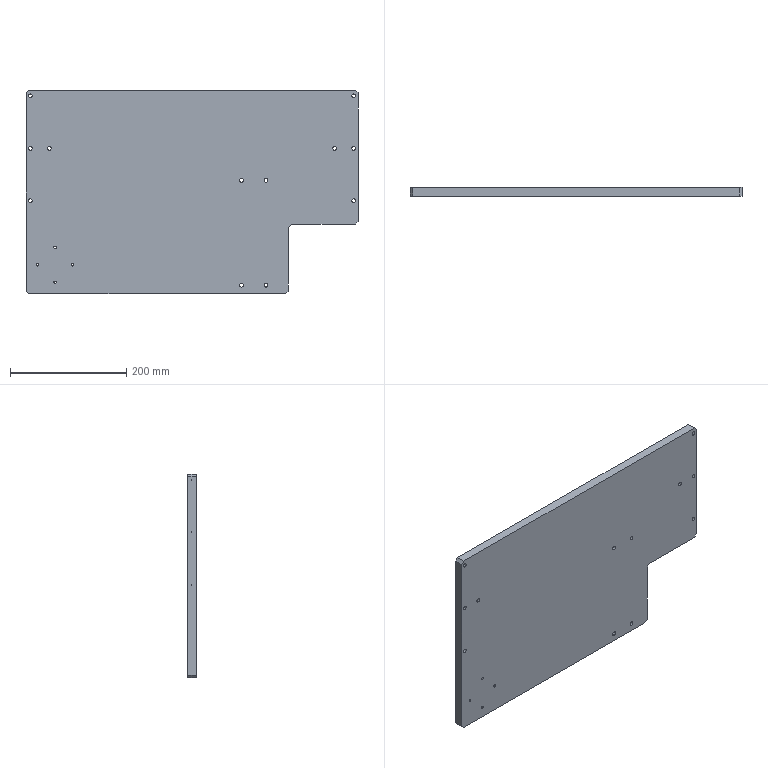Part | SolidWorks | features HoleWzd 4, Chamfer 2, Cut 1, Extrusion 1, Fillet 1 | 1 solid | 70 faces | box 570 x 15 x 350 mm | volume 2765655 mm3 | cylinder 49 | plane 21 | commonest cylinder face diameters 6.6 x16 11 x16 4.2 x8 6.8 x8 20 x1